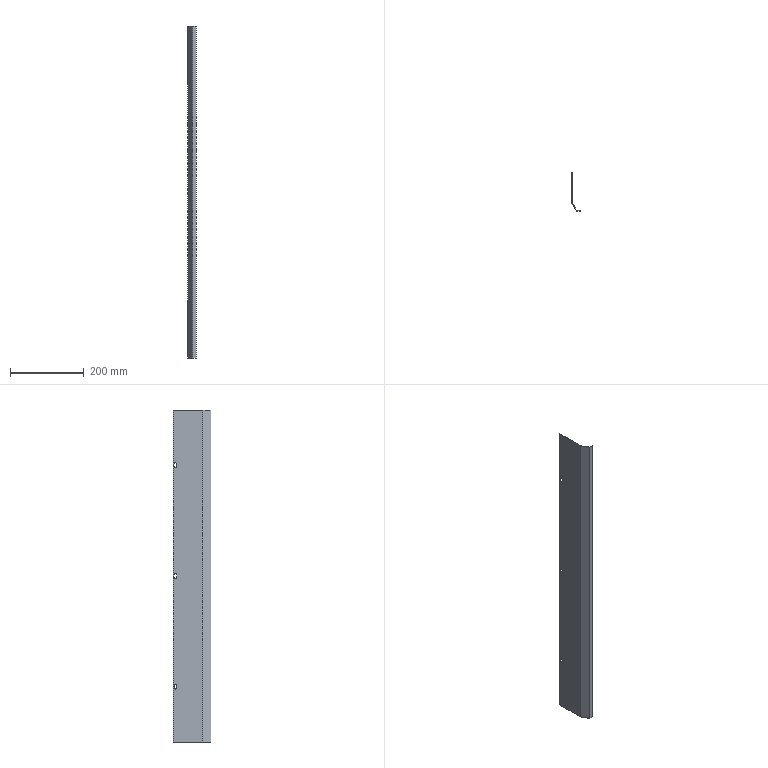Part | 1 solid | 37 faces | box 23.5 x 102.651 x 900 mm | volume 103908 mm3 | plane 24 | cylinder 13 | commonest cylinder face diameters 7 x6 6 x3 1 x2 3 x2
STEP:
#1=CARTESIAN_POINT('',(0.,-3.,-296.5));
#2=VERTEX_POINT('',#1);
#3=CARTESIAN_POINT('',(0.,-6.,-293.5));
#4=VERTEX_POINT('',#3);
#5=CARTESIAN_POINT('',(0.,-6.,-296.5));
#6=DIRECTION('',(1.,0.,0.));
#7=DIRECTION('',(0.,1.,0.));
#8=AXIS2_PLACEMENT_3D('',#5,#6,#7);
#9=CIRCLE('',#8,3.);
#10=EDGE_CURVE('',#2,#4,#9,.T.);
#11=ORIENTED_EDGE('',*,*,#10,.T.);
#12=CARTESIAN_POINT('',(-1.,-6.,-293.5));
#13=VERTEX_POINT('',#12);
#14=CARTESIAN_POINT('',(9.,-6.,-293.5));
#15=DIRECTION('',(-1.,0.,0.));
#16=VECTOR('',#15,1000.);
#17=LINE('',#14,#16);
#18=EDGE_CURVE('',#4,#13,#17,.T.);
#19=ORIENTED_EDGE('',*,*,#18,.T.);
#20=CARTESIAN_POINT('',(-1.,-3.,-296.5));
#21=VERTEX_POINT('',#20);
#22=CARTESIAN_POINT('',(-1.,-6.,-296.5));
#23=DIRECTION('',(-1.,0.,0.));
#24=DIRECTION('',(0.,0.,1.));
#25=AXIS2_PLACEMENT_3D('',#22,#23,#24);
#26=CIRCLE('',#25,3.);
#27=EDGE_CURVE('',#13,#21,#26,.T.);
#28=ORIENTED_EDGE('',*,*,#27,.T.);
#29=CARTESIAN_POINT('',(9.,-3.,-296.5));
#30=DIRECTION('',(-1.,0.,0.));
#31=VECTOR('',#30,1000.);
#32=LINE('',#29,#31);
#33=EDGE_CURVE('',#2,#21,#32,.T.);
#34=ORIENTED_EDGE('',*,*,#33,.F.);
#35=EDGE_LOOP('',(#11,#19,#28,#34));
#36=FACE_OUTER_BOUND('',#35,.T.);
#37=CARTESIAN_POINT('',(9.,-6.,-296.5));
#38=DIRECTION('',(-1.,0.,0.));
#39=DIRECTION('',(0.,0.,1.));
#40=AXIS2_PLACEMENT_3D('',#37,#38,#39);
#41=CYLINDRICAL_SURFACE('',#40,3.);
#42=ADVANCED_FACE('',(#36),#41,.F.);
#43=CARTESIAN_POINT('',(0.,-2.5,303.5));
#44=VERTEX_POINT('',#43);
#45=CARTESIAN_POINT('',(0.,-6.,307.));
#46=VERTEX_POINT('',#45);
#47=CARTESIAN_POINT('',(0.,-6.,303.5));
#48=DIRECTION('',(1.,0.,0.));
#49=DIRECTION('',(0.,1.,0.));
#50=AXIS2_PLACEMENT_3D('',#47,#48,#49);
#51=CIRCLE('',#50,3.5);
#52=EDGE_CURVE('',#44,#46,#51,.T.);
#53=ORIENTED_EDGE('',*,*,#52,.T.);
#54=CARTESIAN_POINT('',(-1.,-6.,307.));
#55=VERTEX_POINT('',#54);
#56=CARTESIAN_POINT('',(9.,-6.,307.));
#57=DIRECTION('',(-1.,0.,0.));
#58=VECTOR('',#57,1000.);
#59=LINE('',#56,#58);
#60=EDGE_CURVE('',#46,#55,#59,.T.);
#61=ORIENTED_EDGE('',*,*,#60,.T.);
#62=CARTESIAN_POINT('',(-1.,-2.5,303.5));
#63=VERTEX_POINT('',#62);
#64=CARTESIAN_POINT('',(-1.,-6.,303.5));
#65=DIRECTION('',(-1.,0.,0.));
#66=DIRECTION('',(0.,0.,1.));
#67=AXIS2_PLACEMENT_3D('',#64,#65,#66);
#68=CIRCLE('',#67,3.5);
#69=EDGE_CURVE('',#55,#63,#68,.T.);
#70=ORIENTED_EDGE('',*,*,#69,.T.);
#71=CARTESIAN_POINT('',(9.,-2.5,303.5));
#72=DIRECTION('',(-1.,0.,0.));
#73=VECTOR('',#72,1000.);
#74=LINE('',#71,#73);
#75=EDGE_CURVE('',#44,#63,#74,.T.);
#76=ORIENTED_EDGE('',*,*,#75,.F.);
#77=EDGE_LOOP('',(#53,#61,#70,#76));
#78=FACE_OUTER_BOUND('',#77,.T.);
#79=CARTESIAN_POINT('',(9.,-6.,303.5));
#80=DIRECTION('',(-1.,0.,0.));
#81=DIRECTION('',(0.,0.,1.));
#82=AXIS2_PLACEMENT_3D('',#79,#80,#81);
#83=CYLINDRICAL_SURFACE('',#82,3.5);
#84=ADVANCED_FACE('',(#78),#83,.F.);
#85=CARTESIAN_POINT('',(0.,-2.5,3.5));
#86=VERTEX_POINT('',#85);
#87=CARTESIAN_POINT('',(0.,-6.,7.));
#88=VERTEX_POINT('',#87);
#89=CARTESIAN_POINT('',(0.,-6.,3.5));
#90=DIRECTION('',(1.,0.,0.));
#91=DIRECTION('',(0.,1.,0.));
#92=AXIS2_PLACEMENT_3D('',#89,#90,#91);
#93=CIRCLE('',#92,3.5);
#94=EDGE_CURVE('',#86,#88,#93,.T.);
#95=ORIENTED_EDGE('',*,*,#94,.T.);
#96=CARTESIAN_POINT('',(-1.,-6.,7.));
#97=VERTEX_POINT('',#96);
#98=CARTESIAN_POINT('',(9.,-6.,7.));
#99=DIRECTION('',(-1.,0.,0.));
#100=VECTOR('',#99,1000.);
#101=LINE('',#98,#100);
#102=EDGE_CURVE('',#88,#97,#101,.T.);
#103=ORIENTED_EDGE('',*,*,#102,.T.);
#104=CARTESIAN_POINT('',(-1.,-2.5,3.5));
#105=VERTEX_POINT('',#104);
#106=CARTESIAN_POINT('',(-1.,-6.,3.5));
#107=DIRECTION('',(-1.,0.,0.));
#108=DIRECTION('',(0.,0.,1.));
#109=AXIS2_PLACEMENT_3D('',#106,#107,#108);
#110=CIRCLE('',#109,3.5);
#111=EDGE_CURVE('',#97,#105,#110,.T.);
#112=ORIENTED_EDGE('',*,*,#111,.T.);
#113=CARTESIAN_POINT('',(9.,-2.5,3.5));
#114=DIRECTION('',(-1.,0.,0.));
#115=VECTOR('',#114,1000.);
#116=LINE('',#113,#115);
#117=EDGE_CURVE('',#86,#105,#116,.T.);
#118=ORIENTED_EDGE('',*,*,#117,.F.);
#119=EDGE_LOOP('',(#95,#103,#112,#118));
#120=FACE_OUTER_BOUND('',#119,.T.);
#121=CARTESIAN_POINT('',(9.,-6.,3.5));
#122=DIRECTION('',(-1.,0.,0.));
#123=DIRECTION('',(0.,0.,1.));
#124=AXIS2_PLACEMENT_3D('',#121,#122,#123);
#125=CYLINDRICAL_SURFACE('',#124,3.5);
#126=ADVANCED_FACE('',(#120),#125,.F.);
#127=CARTESIAN_POINT('',(0.06699,-80.116,450.));
#128=VERTEX_POINT('',#127);
#129=CARTESIAN_POINT('',(-0.799,-80.616,450.));
#130=VERTEX_POINT('',#129);
#131=CARTESIAN_POINT('',(0.06699,-80.116,450.));
#132=DIRECTION('',(-0.866,-0.5,0.));
#133=VECTOR('',#132,1000.);
#134=LINE('',#131,#133);
#135=EDGE_CURVE('',#128,#130,#134,.T.);
#136=ORIENTED_EDGE('',*,*,#135,.F.);
#137=CARTESIAN_POINT('',(0.,-79.866,450.));
#138=VERTEX_POINT('',#137);
#139=CARTESIAN_POINT('',(0.5,-79.866,450.));
#140=DIRECTION('',(0.,0.,1.));
#141=DIRECTION('',(-1.,0.,0.));
#142=AXIS2_PLACEMENT_3D('',#139,#140,#141);
#143=CIRCLE('',#142,0.5);
#144=EDGE_CURVE('',#138,#128,#143,.T.);
#145=ORIENTED_EDGE('',*,*,#144,.F.);
#146=CARTESIAN_POINT('',(-1.,-79.866,450.));
#147=VERTEX_POINT('',#146);
#148=CARTESIAN_POINT('',(-1.,-79.866,450.));
#149=DIRECTION('',(1.,0.,0.));
#150=VECTOR('',#149,1000.);
#151=LINE('',#148,#150);
#152=EDGE_CURVE('',#147,#138,#151,.T.);
#153=ORIENTED_EDGE('',*,*,#152,.F.);
#154=CARTESIAN_POINT('',(0.5,-79.866,450.));
#155=DIRECTION('',(0.,0.,1.));
#156=DIRECTION('',(1.,0.,0.));
#157=AXIS2_PLACEMENT_3D('',#154,#155,#156);
#158=CIRCLE('',#157,1.5);
#159=EDGE_CURVE('',#147,#130,#158,.T.);
#160=ORIENTED_EDGE('',*,*,#159,.T.);
#161=EDGE_LOOP('',(#136,#145,#153,#160));
#162=FACE_OUTER_BOUND('',#161,.T.);
#163=CARTESIAN_POINT('',(0.06699,-80.116,450.));
#164=DIRECTION('',(0.,0.,1.));
#165=DIRECTION('',(1.,0.,0.));
#166=AXIS2_PLACEMENT_3D('',#163,#164,#165);
#167=PLANE('',#166);
#168=ADVANCED_FACE('',(#162),#167,.T.);
#169=CARTESIAN_POINT('',(12.356,-101.401,450.));
#170=VERTEX_POINT('',#169);
#171=CARTESIAN_POINT('',(0.,-80.,450.));
#172=DIRECTION('',(0.5,-0.866,0.));
#173=VECTOR('',#172,1000.);
#174=LINE('',#171,#173);
#175=EDGE_CURVE('',#128,#170,#174,.T.);
#176=ORIENTED_EDGE('',*,*,#175,.F.);
#177=ORIENTED_EDGE('',*,*,#135,.T.);
#178=CARTESIAN_POINT('',(11.49,-101.901,450.));
#179=VERTEX_POINT('',#178);
#180=CARTESIAN_POINT('',(-0.866,-80.5,450.));
#181=DIRECTION('',(0.5,-0.866,0.));
#182=VECTOR('',#181,1000.);
#183=LINE('',#180,#182);
#184=EDGE_CURVE('',#130,#179,#183,.T.);
#185=ORIENTED_EDGE('',*,*,#184,.T.);
#186=CARTESIAN_POINT('',(11.49,-101.901,450.));
#187=DIRECTION('',(0.866,0.5,0.));
#188=VECTOR('',#187,1000.);
#189=LINE('',#186,#188);
#190=EDGE_CURVE('',#179,#170,#189,.T.);
#191=ORIENTED_EDGE('',*,*,#190,.T.);
#192=EDGE_LOOP('',(#176,#177,#185,#191));
#193=FACE_OUTER_BOUND('',#192,.T.);
#194=CARTESIAN_POINT('',(-1.,-79.866,450.));
#195=DIRECTION('',(0.,0.,1.));
#196=DIRECTION('',(1.,0.,0.));
#197=AXIS2_PLACEMENT_3D('',#194,#195,#196);
#198=PLANE('',#197);
#199=ADVANCED_FACE('',(#193),#198,.T.);
#200=CARTESIAN_POINT('',(0.,-79.866,-450.));
#201=VERTEX_POINT('',#200);
#202=CARTESIAN_POINT('',(-1.,-79.866,-450.));
#203=VERTEX_POINT('',#202);
#204=CARTESIAN_POINT('',(0.,-79.866,-450.));
#205=DIRECTION('',(-1.,0.,0.));
#206=VECTOR('',#205,1000.);
#207=LINE('',#204,#206);
#208=EDGE_CURVE('',#201,#203,#207,.T.);
#209=ORIENTED_EDGE('',*,*,#208,.F.);
#210=CARTESIAN_POINT('',(0.06699,-80.116,-450.));
#211=VERTEX_POINT('',#210);
#212=CARTESIAN_POINT('',(0.5,-79.866,-450.));
#213=DIRECTION('',(0.,0.,1.));
#214=DIRECTION('',(-1.,0.,0.));
#215=AXIS2_PLACEMENT_3D('',#212,#213,#214);
#216=CIRCLE('',#215,0.5);
#217=EDGE_CURVE('',#201,#211,#216,.T.);
#218=ORIENTED_EDGE('',*,*,#217,.T.);
#219=CARTESIAN_POINT('',(-0.799,-80.616,-450.));
#220=VERTEX_POINT('',#219);
#221=CARTESIAN_POINT('',(-0.799,-80.616,-450.));
#222=DIRECTION('',(0.866,0.5,0.));
#223=VECTOR('',#222,1000.);
#224=LINE('',#221,#223);
#225=EDGE_CURVE('',#220,#211,#224,.T.);
#226=ORIENTED_EDGE('',*,*,#225,.F.);
#227=CARTESIAN_POINT('',(0.5,-79.866,-450.));
#228=DIRECTION('',(0.,0.,1.));
#229=DIRECTION('',(1.,0.,0.));
#230=AXIS2_PLACEMENT_3D('',#227,#228,#229);
#231=CIRCLE('',#230,1.5);
#232=EDGE_CURVE('',#203,#220,#231,.T.);
#233=ORIENTED_EDGE('',*,*,#232,.F.);
#234=EDGE_LOOP('',(#209,#218,#226,#233));
#235=FACE_OUTER_BOUND('',#234,.T.);
#236=CARTESIAN_POINT('',(0.,-79.866,-450.));
#237=DIRECTION('',(0.,0.,-1.));
#238=DIRECTION('',(-1.,0.,0.));
#239=AXIS2_PLACEMENT_3D('',#236,#237,#238);
#240=PLANE('',#239);
#241=ADVANCED_FACE('',(#235),#240,.T.);
#242=CARTESIAN_POINT('',(0.,0.,-450.));
#243=VERTEX_POINT('',#242);
#244=CARTESIAN_POINT('',(0.,0.,-450.));
#245=DIRECTION('',(0.,-1.,0.));
#246=VECTOR('',#245,1000.);
#247=LINE('',#244,#246);
#248=EDGE_CURVE('',#243,#201,#247,.T.);
#249=ORIENTED_EDGE('',*,*,#248,.T.);
#250=ORIENTED_EDGE('',*,*,#208,.T.);
#251=CARTESIAN_POINT('',(-1.,0.,-450.));
#252=VERTEX_POINT('',#251);
#253=CARTESIAN_POINT('',(-1.,0.,-450.));
#254=DIRECTION('',(0.,-1.,0.));
#255=VECTOR('',#254,1000.);
#256=LINE('',#253,#255);
#257=EDGE_CURVE('',#252,#203,#256,.T.);
#258=ORIENTED_EDGE('',*,*,#257,.F.);
#259=CARTESIAN_POINT('',(-1.,0.,-450.));
#260=DIRECTION('',(1.,0.,0.));
#261=VECTOR('',#260,1000.);
#262=LINE('',#259,#261);
#263=EDGE_CURVE('',#252,#243,#262,.T.);
#264=ORIENTED_EDGE('',*,*,#263,.T.);
#265=EDGE_LOOP('',(#249,#250,#258,#264));
#266=FACE_OUTER_BOUND('',#265,.T.);
#267=CARTESIAN_POINT('',(-0.799,-80.616,-450.));
#268=DIRECTION('',(0.,0.,-1.));
#269=DIRECTION('',(-1.,0.,0.));
#270=AXIS2_PLACEMENT_3D('',#267,#268,#269);
#271=PLANE('',#270);
#272=ADVANCED_FACE('',(#266),#271,.T.);
#273=CARTESIAN_POINT('',(12.789,-101.651,450.));
#274=VERTEX_POINT('',#273);
#275=CARTESIAN_POINT('',(12.789,-102.651,450.));
#276=VERTEX_POINT('',#275);
#277=CARTESIAN_POINT('',(12.789,-101.651,450.));
#278=DIRECTION('',(0.,-1.,0.));
#279=VECTOR('',#278,1000.);
#280=LINE('',#277,#279);
#281=EDGE_CURVE('',#274,#276,#280,.T.);
#282=ORIENTED_EDGE('',*,*,#281,.F.);
#283=CARTESIAN_POINT('',(12.789,-101.151,450.));
#284=DIRECTION('',(0.,0.,1.));
#285=DIRECTION('',(-1.,0.,0.));
#286=AXIS2_PLACEMENT_3D('',#283,#284,#285);
#287=CIRCLE('',#286,0.5);
#288=EDGE_CURVE('',#170,#274,#287,.T.);
#289=ORIENTED_EDGE('',*,*,#288,.F.);
#290=ORIENTED_EDGE('',*,*,#190,.F.);
#291=CARTESIAN_POINT('',(12.789,-101.151,450.));
#292=DIRECTION('',(0.,0.,1.));
#293=DIRECTION('',(1.,0.,0.));
#294=AXIS2_PLACEMENT_3D('',#291,#292,#293);
#295=CIRCLE('',#294,1.5);
#296=EDGE_CURVE('',#179,#276,#295,.T.);
#297=ORIENTED_EDGE('',*,*,#296,.T.);
#298=EDGE_LOOP('',(#282,#289,#290,#297));
#299=FACE_OUTER_BOUND('',#298,.T.);
#300=CARTESIAN_POINT('',(12.789,-101.651,450.));
#301=DIRECTION('',(0.,0.,1.));
#302=DIRECTION('',(1.,0.,0.));
#303=AXIS2_PLACEMENT_3D('',#300,#301,#302);
#304=PLANE('',#303);
#305=ADVANCED_FACE('',(#299),#304,.T.);
#306=CARTESIAN_POINT('',(22.5,-101.651,450.));
#307=VERTEX_POINT('',#306);
#308=CARTESIAN_POINT('',(12.5,-101.651,450.));
#309=DIRECTION('',(1.,0.,0.));
#310=VECTOR('',#309,1000.);
#311=LINE('',#308,#310);
#312=EDGE_CURVE('',#274,#307,#311,.T.);
#313=ORIENTED_EDGE('',*,*,#312,.F.);
#314=ORIENTED_EDGE('',*,*,#281,.T.);
#315=CARTESIAN_POINT('',(22.5,-102.651,450.));
#316=VERTEX_POINT('',#315);
#317=CARTESIAN_POINT('',(12.5,-102.651,450.));
#318=DIRECTION('',(1.,0.,0.));
#319=VECTOR('',#318,1000.);
#320=LINE('',#317,#319);
#321=EDGE_CURVE('',#276,#316,#320,.T.);
#322=ORIENTED_EDGE('',*,*,#321,.T.);
#323=CARTESIAN_POINT('',(22.5,-101.651,450.));
#324=DIRECTION('',(0.,-1.,0.));
#325=VECTOR('',#324,1000.);
#326=LINE('',#323,#325);
#327=EDGE_CURVE('',#307,#316,#326,.T.);
#328=ORIENTED_EDGE('',*,*,#327,.F.);
#329=EDGE_LOOP('',(#313,#314,#322,#328));
#330=FACE_OUTER_BOUND('',#329,.T.);
#331=CARTESIAN_POINT('',(11.49,-101.901,450.));
#332=DIRECTION('',(0.,0.,1.));
#333=DIRECTION('',(1.,0.,0.));
#334=AXIS2_PLACEMENT_3D('',#331,#332,#333);
#335=PLANE('',#334);
#336=ADVANCED_FACE('',(#330),#335,.T.);
#337=CARTESIAN_POINT('',(12.356,-101.401,-450.));
#338=VERTEX_POINT('',#337);
#339=CARTESIAN_POINT('',(11.49,-101.901,-450.));
#340=VERTEX_POINT('',#339);
#341=CARTESIAN_POINT('',(12.356,-101.401,-450.));
#342=DIRECTION('',(-0.866,-0.5,0.));
#343=VECTOR('',#342,1000.);
#344=LINE('',#341,#343);
#345=EDGE_CURVE('',#338,#340,#344,.T.);
#346=ORIENTED_EDGE('',*,*,#345,.F.);
#347=CARTESIAN_POINT('',(12.789,-101.651,-450.));
#348=VERTEX_POINT('',#347);
#349=CARTESIAN_POINT('',(12.789,-101.151,-450.));
#350=DIRECTION('',(0.,0.,1.));
#351=DIRECTION('',(-1.,0.,0.));
#352=AXIS2_PLACEMENT_3D('',#349,#350,#351);
#353=CIRCLE('',#352,0.5);
#354=EDGE_CURVE('',#338,#348,#353,.T.);
#355=ORIENTED_EDGE('',*,*,#354,.T.);
#356=CARTESIAN_POINT('',(12.789,-102.651,-450.));
#357=VERTEX_POINT('',#356);
#358=CARTESIAN_POINT('',(12.789,-102.651,-450.));
#359=DIRECTION('',(0.,1.,0.));
#360=VECTOR('',#359,1000.);
#361=LINE('',#358,#360);
#362=EDGE_CURVE('',#357,#348,#361,.T.);
#363=ORIENTED_EDGE('',*,*,#362,.F.);
#364=CARTESIAN_POINT('',(12.789,-101.151,-450.));
#365=DIRECTION('',(0.,0.,1.));
#366=DIRECTION('',(1.,0.,0.));
#367=AXIS2_PLACEMENT_3D('',#364,#365,#366);
#368=CIRCLE('',#367,1.5);
#369=EDGE_CURVE('',#340,#357,#368,.T.);
#370=ORIENTED_EDGE('',*,*,#369,.F.);
#371=EDGE_LOOP('',(#346,#355,#363,#370));
#372=FACE_OUTER_BOUND('',#371,.T.);
#373=CARTESIAN_POINT('',(12.356,-101.401,-450.));
#374=DIRECTION('',(0.,0.,-1.));
#375=DIRECTION('',(-1.,0.,0.));
#376=AXIS2_PLACEMENT_3D('',#373,#374,#375);
#377=PLANE('',#376);
#378=ADVANCED_FACE('',(#372),#377,.T.);
#379=CARTESIAN_POINT('',(0.,-80.,-450.));
#380=DIRECTION('',(0.5,-0.866,0.));
#381=VECTOR('',#380,1000.);
#382=LINE('',#379,#381);
#383=EDGE_CURVE('',#211,#338,#382,.T.);
#384=ORIENTED_EDGE('',*,*,#383,.T.);
#385=ORIENTED_EDGE('',*,*,#345,.T.);
#386=CARTESIAN_POINT('',(-0.866,-80.5,-450.));
#387=DIRECTION('',(0.5,-0.866,0.));
#388=VECTOR('',#387,1000.);
#389=LINE('',#386,#388);
#390=EDGE_CURVE('',#220,#340,#389,.T.);
#391=ORIENTED_EDGE('',*,*,#390,.F.);
#392=ORIENTED_EDGE('',*,*,#225,.T.);
#393=EDGE_LOOP('',(#384,#385,#391,#392));
#394=FACE_OUTER_BOUND('',#393,.T.);
#395=CARTESIAN_POINT('',(12.789,-102.651,-450.));
#396=DIRECTION('',(0.,0.,-1.));
#397=DIRECTION('',(-1.,0.,0.));
#398=AXIS2_PLACEMENT_3D('',#395,#396,#397);
#399=PLANE('',#398);
#400=ADVANCED_FACE('',(#394),#399,.T.);
#401=CARTESIAN_POINT('',(22.5,-102.651,-450.));
#402=VERTEX_POINT('',#401);
#403=CARTESIAN_POINT('',(12.5,-102.651,-450.));
#404=DIRECTION('',(1.,0.,0.));
#405=VECTOR('',#404,1000.);
#406=LINE('',#403,#405);
#407=EDGE_CURVE('',#357,#402,#406,.T.);
#408=ORIENTED_EDGE('',*,*,#407,.T.);
#409=CARTESIAN_POINT('',(22.5,-102.651,450.));
#410=DIRECTION('',(0.,0.,-1.));
#411=VECTOR('',#410,1000.);
#412=LINE('',#409,#411);
#413=EDGE_CURVE('',#316,#402,#412,.T.);
#414=ORIENTED_EDGE('',*,*,#413,.F.);
#415=ORIENTED_EDGE('',*,*,#321,.F.);
#416=CARTESIAN_POINT('',(12.789,-102.651,450.));
#417=DIRECTION('',(0.,0.,-1.));
#418=VECTOR('',#417,1000.);
#419=LINE('',#416,#418);
#420=EDGE_CURVE('',#276,#357,#419,.T.);
#421=ORIENTED_EDGE('',*,*,#420,.T.);
#422=EDGE_LOOP('',(#408,#414,#415,#421));
#423=FACE_OUTER_BOUND('',#422,.T.);
#424=CARTESIAN_POINT('',(12.5,-102.651,450.));
#425=DIRECTION('',(0.,1.,0.));
#426=DIRECTION('',(0.,0.,1.));
#427=AXIS2_PLACEMENT_3D('',#424,#425,#426);
#428=PLANE('',#427);
#429=ADVANCED_FACE('',(#423),#428,.F.);
#430=CARTESIAN_POINT('',(22.5,-101.651,-450.));
#431=VERTEX_POINT('',#430);
#432=CARTESIAN_POINT('',(22.5,-101.651,-450.));
#433=DIRECTION('',(0.,-1.,0.));
#434=VECTOR('',#433,1000.);
#435=LINE('',#432,#434);
#436=EDGE_CURVE('',#431,#402,#435,.T.);
#437=ORIENTED_EDGE('',*,*,#436,.F.);
#438=CARTESIAN_POINT('',(22.5,-101.651,450.));
#439=DIRECTION('',(0.,0.,-1.));
#440=VECTOR('',#439,1000.);
#441=LINE('',#438,#440);
#442=EDGE_CURVE('',#307,#431,#441,.T.);
#443=ORIENTED_EDGE('',*,*,#442,.F.);
#444=ORIENTED_EDGE('',*,*,#327,.T.);
#445=ORIENTED_EDGE('',*,*,#413,.T.);
#446=EDGE_LOOP('',(#437,#443,#444,#445));
#447=FACE_OUTER_BOUND('',#446,.T.);
#448=CARTESIAN_POINT('',(22.5,-101.651,450.));
#449=DIRECTION('',(1.,0.,0.));
#450=DIRECTION('',(0.,0.,-1.));
#451=AXIS2_PLACEMENT_3D('',#448,#449,#450);
#452=PLANE('',#451);
#453=ADVANCED_FACE('',(#447),#452,.T.);
#454=CARTESIAN_POINT('',(12.5,-101.651,-450.));
#455=DIRECTION('',(1.,0.,0.));
#456=VECTOR('',#455,1000.);
#457=LINE('',#454,#456);
#458=EDGE_CURVE('',#348,#431,#457,.T.);
#459=ORIENTED_EDGE('',*,*,#458,.F.);
#460=CARTESIAN_POINT('',(12.789,-101.651,450.));
#461=DIRECTION('',(0.,0.,-1.));
#462=VECTOR('',#461,1000.);
#463=LINE('',#460,#462);
#464=EDGE_CURVE('',#274,#348,#463,.T.);
#465=ORIENTED_EDGE('',*,*,#464,.F.);
#466=ORIENTED_EDGE('',*,*,#312,.T.);
#467=ORIENTED_EDGE('',*,*,#442,.T.);
#468=EDGE_LOOP('',(#459,#465,#466,#467));
#469=FACE_OUTER_BOUND('',#468,.T.);
#470=CARTESIAN_POINT('',(12.5,-101.651,450.));
#471=DIRECTION('',(0.,1.,0.));
#472=DIRECTION('',(0.,0.,1.));
#473=AXIS2_PLACEMENT_3D('',#470,#471,#472);
#474=PLANE('',#473);
#475=ADVANCED_FACE('',(#469),#474,.T.);
#476=ORIENTED_EDGE('',*,*,#354,.F.);
#477=CARTESIAN_POINT('',(12.356,-101.401,450.));
#478=DIRECTION('',(0.,0.,-1.));
#479=VECTOR('',#478,1000.);
#480=LINE('',#477,#479);
#481=EDGE_CURVE('',#170,#338,#480,.T.);
#482=ORIENTED_EDGE('',*,*,#481,.F.);
#483=ORIENTED_EDGE('',*,*,#288,.T.);
#484=ORIENTED_EDGE('',*,*,#464,.T.);
#485=EDGE_LOOP('',(#476,#482,#483,#484));
#486=FACE_OUTER_BOUND('',#485,.T.);
#487=CARTESIAN_POINT('',(12.789,-101.151,450.));
#488=DIRECTION('',(0.,0.,-1.));
#489=DIRECTION('',(-1.,0.,0.));
#490=AXIS2_PLACEMENT_3D('',#487,#488,#489);
#491=CYLINDRICAL_SURFACE('',#490,0.5);
#492=ADVANCED_FACE('',(#486),#491,.F.);
#493=ORIENTED_EDGE('',*,*,#383,.F.);
#494=CARTESIAN_POINT('',(0.06699,-80.116,450.));
#495=DIRECTION('',(0.,0.,-1.));
#496=VECTOR('',#495,1000.);
#497=LINE('',#494,#496);
#498=EDGE_CURVE('',#128,#211,#497,.T.);
#499=ORIENTED_EDGE('',*,*,#498,.F.);
#500=ORIENTED_EDGE('',*,*,#175,.T.);
#501=ORIENTED_EDGE('',*,*,#481,.T.);
#502=EDGE_LOOP('',(#493,#499,#500,#501));
#503=FACE_OUTER_BOUND('',#502,.T.);
#504=CARTESIAN_POINT('',(0.,-80.,450.));
#505=DIRECTION('',(0.866,0.5,0.));
#506=DIRECTION('',(-0.5,0.866,0.));
#507=AXIS2_PLACEMENT_3D('',#504,#505,#506);
#508=PLANE('',#507);
#509=ADVANCED_FACE('',(#503),#508,.T.);
#510=ORIENTED_EDGE('',*,*,#217,.F.);
#511=CARTESIAN_POINT('',(0.,-79.866,450.));
#512=DIRECTION('',(0.,0.,-1.));
#513=VECTOR('',#512,1000.);
#514=LINE('',#511,#513);
#515=EDGE_CURVE('',#138,#201,#514,.T.);
#516=ORIENTED_EDGE('',*,*,#515,.F.);
#517=ORIENTED_EDGE('',*,*,#144,.T.);
#518=ORIENTED_EDGE('',*,*,#498,.T.);
#519=EDGE_LOOP('',(#510,#516,#517,#518));
#520=FACE_OUTER_BOUND('',#519,.T.);
#521=CARTESIAN_POINT('',(0.5,-79.866,450.));
#522=DIRECTION('',(0.,0.,-1.));
#523=DIRECTION('',(-1.,0.,0.));
#524=AXIS2_PLACEMENT_3D('',#521,#522,#523);
#525=CYLINDRICAL_SURFACE('',#524,0.5);
#526=ADVANCED_FACE('',(#520),#525,.F.);
#527=CARTESIAN_POINT('',(0.,-9.,-303.5));
#528=VERTEX_POINT('',#527);
#529=CARTESIAN_POINT('',(0.,-3.,-303.5));
#530=VERTEX_POINT('',#529);
#531=CARTESIAN_POINT('',(0.,-6.,-303.5));
#532=DIRECTION('',(1.,0.,0.));
#533=DIRECTION('',(0.,1.,0.));
#534=AXIS2_PLACEMENT_3D('',#531,#532,#533);
#535=CIRCLE('',#534,3.);
#536=EDGE_CURVE('',#528,#530,#535,.T.);
#537=ORIENTED_EDGE('',*,*,#536,.F.);
#538=CARTESIAN_POINT('',(0.,-9.,-296.5));
#539=VERTEX_POINT('',#538);
#540=CARTESIAN_POINT('',(0.,-9.,450.));
#541=DIRECTION('',(0.,0.,-1.));
#542=VECTOR('',#541,1000.);
#543=LINE('',#540,#542);
#544=EDGE_CURVE('',#539,#528,#543,.T.);
#545=ORIENTED_EDGE('',*,*,#544,.F.);
#546=CARTESIAN_POINT('',(0.,-6.,-296.5));
#547=DIRECTION('',(1.,0.,0.));
#548=DIRECTION('',(0.,1.,0.));
#549=AXIS2_PLACEMENT_3D('',#546,#547,#548);
#550=CIRCLE('',#549,3.);
#551=EDGE_CURVE('',#4,#539,#550,.T.);
#552=ORIENTED_EDGE('',*,*,#551,.F.);
#553=ORIENTED_EDGE('',*,*,#10,.F.);
#554=CARTESIAN_POINT('',(0.,-3.,450.));
#555=DIRECTION('',(0.,0.,1.));
#556=VECTOR('',#555,1000.);
#557=LINE('',#554,#556);
#558=EDGE_CURVE('',#530,#2,#557,.T.);
#559=ORIENTED_EDGE('',*,*,#558,.F.);
#560=EDGE_LOOP('',(#537,#545,#552,#553,#559));
#561=FACE_BOUND('',#560,.T.);
#562=CARTESIAN_POINT('',(0.,-9.5,296.5));
#563=VERTEX_POINT('',#562);
#564=CARTESIAN_POINT('',(0.,-2.5,296.5));
#565=VERTEX_POINT('',#564);
#566=CARTESIAN_POINT('',(0.,-6.,296.5));
#567=DIRECTION('',(1.,0.,0.));
#568=DIRECTION('',(0.,1.,0.));
#569=AXIS2_PLACEMENT_3D('',#566,#567,#568);
#570=CIRCLE('',#569,3.5);
#571=EDGE_CURVE('',#563,#565,#570,.T.);
#572=ORIENTED_EDGE('',*,*,#571,.F.);
#573=CARTESIAN_POINT('',(0.,-9.5,303.5));
#574=VERTEX_POINT('',#573);
#575=CARTESIAN_POINT('',(0.,-9.5,450.));
#576=DIRECTION('',(0.,0.,-1.));
#577=VECTOR('',#576,1000.);
#578=LINE('',#575,#577);
#579=EDGE_CURVE('',#574,#563,#578,.T.);
#580=ORIENTED_EDGE('',*,*,#579,.F.);
#581=CARTESIAN_POINT('',(0.,-6.,303.5));
#582=DIRECTION('',(1.,0.,0.));
#583=DIRECTION('',(0.,1.,0.));
#584=AXIS2_PLACEMENT_3D('',#581,#582,#583);
#585=CIRCLE('',#584,3.5);
#586=EDGE_CURVE('',#46,#574,#585,.T.);
#587=ORIENTED_EDGE('',*,*,#586,.F.);
#588=ORIENTED_EDGE('',*,*,#52,.F.);
#589=CARTESIAN_POINT('',(0.,-2.5,450.));
#590=DIRECTION('',(0.,0.,1.));
#591=VECTOR('',#590,1000.);
#592=LINE('',#589,#591);
#593=EDGE_CURVE('',#565,#44,#592,.T.);
#594=ORIENTED_EDGE('',*,*,#593,.F.);
#595=EDGE_LOOP('',(#572,#580,#587,#588,#594));
#596=FACE_BOUND('',#595,.T.);
#597=CARTESIAN_POINT('',(0.,-9.5,-3.5));
#598=VERTEX_POINT('',#597);
#599=CARTESIAN_POINT('',(0.,-2.5,-3.5));
#600=VERTEX_POINT('',#599);
#601=CARTESIAN_POINT('',(0.,-6.,-3.5));
#602=DIRECTION('',(1.,0.,0.));
#603=DIRECTION('',(0.,1.,0.));
#604=AXIS2_PLACEMENT_3D('',#601,#602,#603);
#605=CIRCLE('',#604,3.5);
#606=EDGE_CURVE('',#598,#600,#605,.T.);
#607=ORIENTED_EDGE('',*,*,#606,.F.);
#608=CARTESIAN_POINT('',(0.,-9.5,3.5));
#609=VERTEX_POINT('',#608);
#610=CARTESIAN_POINT('',(0.,-9.5,450.));
#611=DIRECTION('',(0.,0.,-1.));
#612=VECTOR('',#611,1000.);
#613=LINE('',#610,#612);
#614=EDGE_CURVE('',#609,#598,#613,.T.);
#615=ORIENTED_EDGE('',*,*,#614,.F.);
#616=CARTESIAN_POINT('',(0.,-6.,3.5));
#617=DIRECTION('',(1.,0.,0.));
#618=DIRECTION('',(0.,1.,0.));
#619=AXIS2_PLACEMENT_3D('',#616,#617,#618);
#620=CIRCLE('',#619,3.5);
#621=EDGE_CURVE('',#88,#609,#620,.T.);
#622=ORIENTED_EDGE('',*,*,#621,.F.);
#623=ORIENTED_EDGE('',*,*,#94,.F.);
#624=CARTESIAN_POINT('',(0.,-2.5,450.));
#625=DIRECTION('',(0.,0.,1.));
#626=VECTOR('',#625,1000.);
#627=LINE('',#624,#626);
#628=EDGE_CURVE('',#600,#86,#627,.T.);
#629=ORIENTED_EDGE('',*,*,#628,.F.);
#630=EDGE_LOOP('',(#607,#615,#622,#623,#629));
#631=FACE_BOUND('',#630,.T.);
#632=ORIENTED_EDGE('',*,*,#248,.F.);
#633=CARTESIAN_POINT('',(0.,0.,450.));
#634=VERTEX_POINT('',#633);
#635=CARTESIAN_POINT('',(0.,0.,450.));
#636=DIRECTION('',(0.,0.,-1.));
#637=VECTOR('',#636,1000.);
#638=LINE('',#635,#637);
#639=EDGE_CURVE('',#634,#243,#638,.T.);
#640=ORIENTED_EDGE('',*,*,#639,.F.);
#641=CARTESIAN_POINT('',(0.,0.,450.));
#642=DIRECTION('',(0.,-1.,0.));
#643=VECTOR('',#642,1000.);
#644=LINE('',#641,#643);
#645=EDGE_CURVE('',#634,#138,#644,.T.);
#646=ORIENTED_EDGE('',*,*,#645,.T.);
#647=ORIENTED_EDGE('',*,*,#515,.T.);
#648=EDGE_LOOP('',(#632,#640,#646,#647));
#649=FACE_OUTER_BOUND('',#648,.T.);
#650=CARTESIAN_POINT('',(0.,0.,450.));
#651=DIRECTION('',(1.,0.,0.));
#652=DIRECTION('',(0.,1.,0.));
#653=AXIS2_PLACEMENT_3D('',#650,#651,#652);
#654=PLANE('',#653);
#655=ADVANCED_FACE('',(#561,#596,#631,#649),#654,.T.);
#656=ORIENTED_EDGE('',*,*,#263,.F.);
#657=CARTESIAN_POINT('',(-1.,0.,450.));
#658=VERTEX_POINT('',#657);
#659=CARTESIAN_POINT('',(-1.,0.,450.));
#660=DIRECTION('',(0.,0.,-1.));
#661=VECTOR('',#660,1000.);
#662=LINE('',#659,#661);
#663=EDGE_CURVE('',#658,#252,#662,.T.);
#664=ORIENTED_EDGE('',*,*,#663,.F.);
#665=CARTESIAN_POINT('',(-1.,0.,450.));
#666=DIRECTION('',(1.,0.,0.));
#667=VECTOR('',#666,1000.);
#668=LINE('',#665,#667);
#669=EDGE_CURVE('',#658,#634,#668,.T.);
#670=ORIENTED_EDGE('',*,*,#669,.T.);
#671=ORIENTED_EDGE('',*,*,#639,.T.);
#672=EDGE_LOOP('',(#656,#664,#670,#671));
#673=FACE_OUTER_BOUND('',#672,.T.);
#674=CARTESIAN_POINT('',(-1.,0.,450.));
#675=DIRECTION('',(0.,1.,0.));
#676=DIRECTION('',(-1.,0.,0.));
#677=AXIS2_PLACEMENT_3D('',#674,#675,#676);
#678=PLANE('',#677);
#679=ADVANCED_FACE('',(#673),#678,.T.);
#680=CARTESIAN_POINT('',(-1.,-9.,-303.5));
#681=VERTEX_POINT('',#680);
#682=CARTESIAN_POINT('',(-1.,-9.,-296.5));
#683=VERTEX_POINT('',#682);
#684=CARTESIAN_POINT('',(-1.,-9.,-303.5));
#685=DIRECTION('',(0.,0.,1.));
#686=VECTOR('',#685,1000.);
#687=LINE('',#684,#686);
#688=EDGE_CURVE('',#681,#683,#687,.T.);
#689=ORIENTED_EDGE('',*,*,#688,.F.);
#690=CARTESIAN_POINT('',(-1.,-3.,-303.5));
#691=VERTEX_POINT('',#690);
#692=CARTESIAN_POINT('',(-1.,-6.,-303.5));
#693=DIRECTION('',(-1.,0.,0.));
#694=DIRECTION('',(0.,0.,1.));
#695=AXIS2_PLACEMENT_3D('',#692,#693,#694);
#696=CIRCLE('',#695,3.);
#697=EDGE_CURVE('',#691,#681,#696,.T.);
#698=ORIENTED_EDGE('',*,*,#697,.F.);
#699=CARTESIAN_POINT('',(-1.,-3.,-303.5));
#700=DIRECTION('',(0.,0.,-1.));
#701=VECTOR('',#700,1000.);
#702=LINE('',#699,#701);
#703=EDGE_CURVE('',#21,#691,#702,.T.);
#704=ORIENTED_EDGE('',*,*,#703,.F.);
#705=ORIENTED_EDGE('',*,*,#27,.F.);
#706=CARTESIAN_POINT('',(-1.,-6.,-296.5));
#707=DIRECTION('',(-1.,0.,0.));
#708=DIRECTION('',(0.,0.,1.));
#709=AXIS2_PLACEMENT_3D('',#706,#707,#708);
#710=CIRCLE('',#709,3.);
#711=EDGE_CURVE('',#683,#13,#710,.T.);
#712=ORIENTED_EDGE('',*,*,#711,.F.);
#713=EDGE_LOOP('',(#689,#698,#704,#705,#712));
#714=FACE_BOUND('',#713,.T.);
#715=CARTESIAN_POINT('',(-1.,-9.5,296.5));
#716=VERTEX_POINT('',#715);
#717=CARTESIAN_POINT('',(-1.,-9.5,303.5));
#718=VERTEX_POINT('',#717);
#719=CARTESIAN_POINT('',(-1.,-9.5,296.5));
#720=DIRECTION('',(0.,0.,1.));
#721=VECTOR('',#720,1000.);
#722=LINE('',#719,#721);
#723=EDGE_CURVE('',#716,#718,#722,.T.);
#724=ORIENTED_EDGE('',*,*,#723,.F.);
#725=CARTESIAN_POINT('',(-1.,-2.5,296.5));
#726=VERTEX_POINT('',#725);
#727=CARTESIAN_POINT('',(-1.,-6.,296.5));
#728=DIRECTION('',(-1.,0.,0.));
#729=DIRECTION('',(0.,0.,1.));
#730=AXIS2_PLACEMENT_3D('',#727,#728,#729);
#731=CIRCLE('',#730,3.5);
#732=EDGE_CURVE('',#726,#716,#731,.T.);
#733=ORIENTED_EDGE('',*,*,#732,.F.);
#734=CARTESIAN_POINT('',(-1.,-2.5,296.5));
#735=DIRECTION('',(0.,0.,-1.));
#736=VECTOR('',#735,1000.);
#737=LINE('',#734,#736);
#738=EDGE_CURVE('',#63,#726,#737,.T.);
#739=ORIENTED_EDGE('',*,*,#738,.F.);
#740=ORIENTED_EDGE('',*,*,#69,.F.);
#741=CARTESIAN_POINT('',(-1.,-6.,303.5));
#742=DIRECTION('',(-1.,0.,0.));
#743=DIRECTION('',(0.,0.,1.));
#744=AXIS2_PLACEMENT_3D('',#741,#742,#743);
#745=CIRCLE('',#744,3.5);
#746=EDGE_CURVE('',#718,#55,#745,.T.);
#747=ORIENTED_EDGE('',*,*,#746,.F.);
#748=EDGE_LOOP('',(#724,#733,#739,#740,#747));
#749=FACE_BOUND('',#748,.T.);
#750=CARTESIAN_POINT('',(-1.,-9.5,-3.5));
#751=VERTEX_POINT('',#750);
#752=CARTESIAN_POINT('',(-1.,-9.5,3.5));
#753=VERTEX_POINT('',#752);
#754=CARTESIAN_POINT('',(-1.,-9.5,-3.5));
#755=DIRECTION('',(0.,0.,1.));
#756=VECTOR('',#755,1000.);
#757=LINE('',#754,#756);
#758=EDGE_CURVE('',#751,#753,#757,.T.);
#759=ORIENTED_EDGE('',*,*,#758,.F.);
#760=CARTESIAN_POINT('',(-1.,-2.5,-3.5));
#761=VERTEX_POINT('',#760);
#762=CARTESIAN_POINT('',(-1.,-6.,-3.5));
#763=DIRECTION('',(-1.,0.,0.));
#764=DIRECTION('',(0.,0.,1.));
#765=AXIS2_PLACEMENT_3D('',#762,#763,#764);
#766=CIRCLE('',#765,3.5);
#767=EDGE_CURVE('',#761,#751,#766,.T.);
#768=ORIENTED_EDGE('',*,*,#767,.F.);
#769=CARTESIAN_POINT('',(-1.,-2.5,-3.5));
#770=DIRECTION('',(0.,0.,-1.));
#771=VECTOR('',#770,1000.);
#772=LINE('',#769,#771);
#773=EDGE_CURVE('',#105,#761,#772,.T.);
#774=ORIENTED_EDGE('',*,*,#773,.F.);
#775=ORIENTED_EDGE('',*,*,#111,.F.);
#776=CARTESIAN_POINT('',(-1.,-6.,3.5));
#777=DIRECTION('',(-1.,0.,0.));
#778=DIRECTION('',(0.,0.,1.));
#779=AXIS2_PLACEMENT_3D('',#776,#777,#778);
#780=CIRCLE('',#779,3.5);
#781=EDGE_CURVE('',#753,#97,#780,.T.);
#782=ORIENTED_EDGE('',*,*,#781,.F.);
#783=EDGE_LOOP('',(#759,#768,#774,#775,#782));
#784=FACE_BOUND('',#783,.T.);
#785=ORIENTED_EDGE('',*,*,#257,.T.);
#786=CARTESIAN_POINT('',(-1.,-79.866,450.));
#787=DIRECTION('',(0.,0.,-1.));
#788=VECTOR('',#787,1000.);
#789=LINE('',#786,#788);
#790=EDGE_CURVE('',#147,#203,#789,.T.);
#791=ORIENTED_EDGE('',*,*,#790,.F.);
#792=CARTESIAN_POINT('',(-1.,0.,450.));
#793=DIRECTION('',(0.,-1.,0.));
#794=VECTOR('',#793,1000.);
#795=LINE('',#792,#794);
#796=EDGE_CURVE('',#658,#147,#795,.T.);
#797=ORIENTED_EDGE('',*,*,#796,.F.);
#798=ORIENTED_EDGE('',*,*,#663,.T.);
#799=EDGE_LOOP('',(#785,#791,#797,#798));
#800=FACE_OUTER_BOUND('',#799,.T.);
#801=CARTESIAN_POINT('',(-1.,0.,450.));
#802=DIRECTION('',(1.,0.,0.));
#803=DIRECTION('',(0.,1.,0.));
#804=AXIS2_PLACEMENT_3D('',#801,#802,#803);
#805=PLANE('',#804);
#806=ADVANCED_FACE('',(#714,#749,#784,#800),#805,.F.);
#807=ORIENTED_EDGE('',*,*,#232,.T.);
#808=CARTESIAN_POINT('',(-0.799,-80.616,450.));
#809=DIRECTION('',(0.,0.,-1.));
#810=VECTOR('',#809,1000.);
#811=LINE('',#808,#810);
#812=EDGE_CURVE('',#130,#220,#811,.T.);
#813=ORIENTED_EDGE('',*,*,#812,.F.);
#814=ORIENTED_EDGE('',*,*,#159,.F.);
#815=ORIENTED_EDGE('',*,*,#790,.T.);
#816=EDGE_LOOP('',(#807,#813,#814,#815));
#817=FACE_OUTER_BOUND('',#816,.T.);
#818=CARTESIAN_POINT('',(0.5,-79.866,450.));
#819=DIRECTION('',(0.,0.,-1.));
#820=DIRECTION('',(-1.,0.,0.));
#821=AXIS2_PLACEMENT_3D('',#818,#819,#820);
#822=CYLINDRICAL_SURFACE('',#821,1.5);
#823=ADVANCED_FACE('',(#817),#822,.T.);
#824=ORIENTED_EDGE('',*,*,#390,.T.);
#825=CARTESIAN_POINT('',(11.49,-101.901,450.));
#826=DIRECTION('',(0.,0.,-1.));
#827=VECTOR('',#826,1000.);
#828=LINE('',#825,#827);
#829=EDGE_CURVE('',#179,#340,#828,.T.);
#830=ORIENTED_EDGE('',*,*,#829,.F.);
#831=ORIENTED_EDGE('',*,*,#184,.F.);
#832=ORIENTED_EDGE('',*,*,#812,.T.);
#833=EDGE_LOOP('',(#824,#830,#831,#832));
#834=FACE_OUTER_BOUND('',#833,.T.);
#835=CARTESIAN_POINT('',(-0.866,-80.5,450.));
#836=DIRECTION('',(0.866,0.5,0.));
#837=DIRECTION('',(-0.5,0.866,0.));
#838=AXIS2_PLACEMENT_3D('',#835,#836,#837);
#839=PLANE('',#838);
#840=ADVANCED_FACE('',(#834),#839,.F.);
#841=ORIENTED_EDGE('',*,*,#369,.T.);
#842=ORIENTED_EDGE('',*,*,#420,.F.);
#843=ORIENTED_EDGE('',*,*,#296,.F.);
#844=ORIENTED_EDGE('',*,*,#829,.T.);
#845=EDGE_LOOP('',(#841,#842,#843,#844));
#846=FACE_OUTER_BOUND('',#845,.T.);
#847=CARTESIAN_POINT('',(12.789,-101.151,450.));
#848=DIRECTION('',(0.,0.,-1.));
#849=DIRECTION('',(-1.,0.,0.));
#850=AXIS2_PLACEMENT_3D('',#847,#848,#849);
#851=CYLINDRICAL_SURFACE('',#850,1.5);
#852=ADVANCED_FACE('',(#846),#851,.T.);
#853=ORIENTED_EDGE('',*,*,#796,.T.);
#854=ORIENTED_EDGE('',*,*,#152,.T.);
#855=ORIENTED_EDGE('',*,*,#645,.F.);
#856=ORIENTED_EDGE('',*,*,#669,.F.);
#857=EDGE_LOOP('',(#853,#854,#855,#856));
#858=FACE_OUTER_BOUND('',#857,.T.);
#859=CARTESIAN_POINT('',(12.789,-101.151,450.));
#860=DIRECTION('',(0.,0.,-1.));
#861=DIRECTION('',(-1.,0.,0.));
#862=AXIS2_PLACEMENT_3D('',#859,#860,#861);
#863=PLANE('',#862);
#864=ADVANCED_FACE('',(#858),#863,.F.);
#865=ORIENTED_EDGE('',*,*,#407,.F.);
#866=ORIENTED_EDGE('',*,*,#362,.T.);
#867=ORIENTED_EDGE('',*,*,#458,.T.);
#868=ORIENTED_EDGE('',*,*,#436,.T.);
#869=EDGE_LOOP('',(#865,#866,#867,#868));
#870=FACE_OUTER_BOUND('',#869,.T.);
#871=CARTESIAN_POINT('',(12.789,-101.151,-450.));
#872=DIRECTION('',(0.,0.,-1.));
#873=DIRECTION('',(-1.,0.,0.));
#874=AXIS2_PLACEMENT_3D('',#871,#872,#873);
#875=PLANE('',#874);
#876=ADVANCED_FACE('',(#870),#875,.T.);
#877=ORIENTED_EDGE('',*,*,#606,.T.);
#878=CARTESIAN_POINT('',(9.,-2.5,-3.5));
#879=DIRECTION('',(-1.,0.,0.));
#880=VECTOR('',#879,1000.);
#881=LINE('',#878,#880);
#882=EDGE_CURVE('',#600,#761,#881,.T.);
#883=ORIENTED_EDGE('',*,*,#882,.T.);
#884=ORIENTED_EDGE('',*,*,#767,.T.);
#885=CARTESIAN_POINT('',(9.,-9.5,-3.5));
#886=DIRECTION('',(-1.,0.,0.));
#887=VECTOR('',#886,1000.);
#888=LINE('',#885,#887);
#889=EDGE_CURVE('',#598,#751,#888,.T.);
#890=ORIENTED_EDGE('',*,*,#889,.F.);
#891=EDGE_LOOP('',(#877,#883,#884,#890));
#892=FACE_OUTER_BOUND('',#891,.T.);
#893=CARTESIAN_POINT('',(9.,-6.,-3.5));
#894=DIRECTION('',(-1.,0.,0.));
#895=DIRECTION('',(0.,0.,1.));
#896=AXIS2_PLACEMENT_3D('',#893,#894,#895);
#897=CYLINDRICAL_SURFACE('',#896,3.5);
#898=ADVANCED_FACE('',(#892),#897,.F.);
#899=ORIENTED_EDGE('',*,*,#628,.T.);
#900=ORIENTED_EDGE('',*,*,#117,.T.);
#901=ORIENTED_EDGE('',*,*,#773,.T.);
#902=ORIENTED_EDGE('',*,*,#882,.F.);
#903=EDGE_LOOP('',(#899,#900,#901,#902));
#904=FACE_OUTER_BOUND('',#903,.T.);
#905=CARTESIAN_POINT('',(9.,-2.5,-3.5));
#906=DIRECTION('',(0.,1.,0.));
#907=DIRECTION('',(0.,0.,1.));
#908=AXIS2_PLACEMENT_3D('',#905,#906,#907);
#909=PLANE('',#908);
#910=ADVANCED_FACE('',(#904),#909,.F.);
#911=ORIENTED_EDGE('',*,*,#102,.F.);
#912=ORIENTED_EDGE('',*,*,#621,.T.);
#913=CARTESIAN_POINT('',(9.,-9.5,3.5));
#914=DIRECTION('',(-1.,0.,0.));
#915=VECTOR('',#914,1000.);
#916=LINE('',#913,#915);
#917=EDGE_CURVE('',#609,#753,#916,.T.);
#918=ORIENTED_EDGE('',*,*,#917,.T.);
#919=ORIENTED_EDGE('',*,*,#781,.T.);
#920=EDGE_LOOP('',(#911,#912,#918,#919));
#921=FACE_OUTER_BOUND('',#920,.T.);
#922=CARTESIAN_POINT('',(9.,-6.,3.5));
#923=DIRECTION('',(-1.,0.,0.));
#924=DIRECTION('',(0.,0.,1.));
#925=AXIS2_PLACEMENT_3D('',#922,#923,#924);
#926=CYLINDRICAL_SURFACE('',#925,3.5);
#927=ADVANCED_FACE('',(#921),#926,.F.);
#928=ORIENTED_EDGE('',*,*,#614,.T.);
#929=ORIENTED_EDGE('',*,*,#889,.T.);
#930=ORIENTED_EDGE('',*,*,#758,.T.);
#931=ORIENTED_EDGE('',*,*,#917,.F.);
#932=EDGE_LOOP('',(#928,#929,#930,#931));
#933=FACE_OUTER_BOUND('',#932,.T.);
#934=CARTESIAN_POINT('',(9.,-9.5,-3.5));
#935=DIRECTION('',(0.,-1.,0.));
#936=DIRECTION('',(0.,0.,-1.));
#937=AXIS2_PLACEMENT_3D('',#934,#935,#936);
#938=PLANE('',#937);
#939=ADVANCED_FACE('',(#933),#938,.F.);
#940=ORIENTED_EDGE('',*,*,#571,.T.);
#941=CARTESIAN_POINT('',(9.,-2.5,296.5));
#942=DIRECTION('',(-1.,0.,0.));
#943=VECTOR('',#942,1000.);
#944=LINE('',#941,#943);
#945=EDGE_CURVE('',#565,#726,#944,.T.);
#946=ORIENTED_EDGE('',*,*,#945,.T.);
#947=ORIENTED_EDGE('',*,*,#732,.T.);
#948=CARTESIAN_POINT('',(9.,-9.5,296.5));
#949=DIRECTION('',(-1.,0.,0.));
#950=VECTOR('',#949,1000.);
#951=LINE('',#948,#950);
#952=EDGE_CURVE('',#563,#716,#951,.T.);
#953=ORIENTED_EDGE('',*,*,#952,.F.);
#954=EDGE_LOOP('',(#940,#946,#947,#953));
#955=FACE_OUTER_BOUND('',#954,.T.);
#956=CARTESIAN_POINT('',(9.,-6.,296.5));
#957=DIRECTION('',(-1.,0.,0.));
#958=DIRECTION('',(0.,0.,1.));
#959=AXIS2_PLACEMENT_3D('',#956,#957,#958);
#960=CYLINDRICAL_SURFACE('',#959,3.5);
#961=ADVANCED_FACE('',(#955),#960,.F.);
#962=ORIENTED_EDGE('',*,*,#593,.T.);
#963=ORIENTED_EDGE('',*,*,#75,.T.);
#964=ORIENTED_EDGE('',*,*,#738,.T.);
#965=ORIENTED_EDGE('',*,*,#945,.F.);
#966=EDGE_LOOP('',(#962,#963,#964,#965));
#967=FACE_OUTER_BOUND('',#966,.T.);
#968=CARTESIAN_POINT('',(9.,-2.5,296.5));
#969=DIRECTION('',(0.,1.,0.));
#970=DIRECTION('',(0.,0.,1.));
#971=AXIS2_PLACEMENT_3D('',#968,#969,#970);
#972=PLANE('',#971);
#973=ADVANCED_FACE('',(#967),#972,.F.);
#974=ORIENTED_EDGE('',*,*,#60,.F.);
#975=ORIENTED_EDGE('',*,*,#586,.T.);
#976=CARTESIAN_POINT('',(9.,-9.5,303.5));
#977=DIRECTION('',(-1.,0.,0.));
#978=VECTOR('',#977,1000.);
#979=LINE('',#976,#978);
#980=EDGE_CURVE('',#574,#718,#979,.T.);
#981=ORIENTED_EDGE('',*,*,#980,.T.);
#982=ORIENTED_EDGE('',*,*,#746,.T.);
#983=EDGE_LOOP('',(#974,#975,#981,#982));
#984=FACE_OUTER_BOUND('',#983,.T.);
#985=CARTESIAN_POINT('',(9.,-6.,303.5));
#986=DIRECTION('',(-1.,0.,0.));
#987=DIRECTION('',(0.,0.,1.));
#988=AXIS2_PLACEMENT_3D('',#985,#986,#987);
#989=CYLINDRICAL_SURFACE('',#988,3.5);
#990=ADVANCED_FACE('',(#984),#989,.F.);
#991=ORIENTED_EDGE('',*,*,#579,.T.);
#992=ORIENTED_EDGE('',*,*,#952,.T.);
#993=ORIENTED_EDGE('',*,*,#723,.T.);
#994=ORIENTED_EDGE('',*,*,#980,.F.);
#995=EDGE_LOOP('',(#991,#992,#993,#994));
#996=FACE_OUTER_BOUND('',#995,.T.);
#997=CARTESIAN_POINT('',(9.,-9.5,296.5));
#998=DIRECTION('',(0.,-1.,0.));
#999=DIRECTION('',(0.,0.,-1.));
#1000=AXIS2_PLACEMENT_3D('',#997,#998,#999);
#1001=PLANE('',#1000);
#1002=ADVANCED_FACE('',(#996),#1001,.F.);
#1003=ORIENTED_EDGE('',*,*,#536,.T.);
#1004=CARTESIAN_POINT('',(9.,-3.,-303.5));
#1005=DIRECTION('',(-1.,0.,0.));
#1006=VECTOR('',#1005,1000.);
#1007=LINE('',#1004,#1006);
#1008=EDGE_CURVE('',#530,#691,#1007,.T.);
#1009=ORIENTED_EDGE('',*,*,#1008,.T.);
#1010=ORIENTED_EDGE('',*,*,#697,.T.);
#1011=CARTESIAN_POINT('',(9.,-9.,-303.5));
#1012=DIRECTION('',(-1.,0.,0.));
#1013=VECTOR('',#1012,1000.);
#1014=LINE('',#1011,#1013);
#1015=EDGE_CURVE('',#528,#681,#1014,.T.);
#1016=ORIENTED_EDGE('',*,*,#1015,.F.);
#1017=EDGE_LOOP('',(#1003,#1009,#1010,#1016));
#1018=FACE_OUTER_BOUND('',#1017,.T.);
#1019=CARTESIAN_POINT('',(9.,-6.,-303.5));
#1020=DIRECTION('',(-1.,0.,0.));
#1021=DIRECTION('',(0.,0.,1.));
#1022=AXIS2_PLACEMENT_3D('',#1019,#1020,#1021);
#1023=CYLINDRICAL_SURFACE('',#1022,3.);
#1024=ADVANCED_FACE('',(#1018),#1023,.F.);
#1025=ORIENTED_EDGE('',*,*,#558,.T.);
#1026=ORIENTED_EDGE('',*,*,#33,.T.);
#1027=ORIENTED_EDGE('',*,*,#703,.T.);
#1028=ORIENTED_EDGE('',*,*,#1008,.F.);
#1029=EDGE_LOOP('',(#1025,#1026,#1027,#1028));
#1030=FACE_OUTER_BOUND('',#1029,.T.);
#1031=CARTESIAN_POINT('',(9.,-3.,-303.5));
#1032=DIRECTION('',(0.,1.,0.));
#1033=DIRECTION('',(0.,0.,1.));
#1034=AXIS2_PLACEMENT_3D('',#1031,#1032,#1033);
#1035=PLANE('',#1034);
#1036=ADVANCED_FACE('',(#1030),#1035,.F.);
#1037=ORIENTED_EDGE('',*,*,#18,.F.);
#1038=ORIENTED_EDGE('',*,*,#551,.T.);
#1039=CARTESIAN_POINT('',(9.,-9.,-296.5));
#1040=DIRECTION('',(-1.,0.,0.));
#1041=VECTOR('',#1040,1000.);
#1042=LINE('',#1039,#1041);
#1043=EDGE_CURVE('',#539,#683,#1042,.T.);
#1044=ORIENTED_EDGE('',*,*,#1043,.T.);
#1045=ORIENTED_EDGE('',*,*,#711,.T.);
#1046=EDGE_LOOP('',(#1037,#1038,#1044,#1045));
#1047=FACE_OUTER_BOUND('',#1046,.T.);
#1048=CARTESIAN_POINT('',(9.,-6.,-296.5));
#1049=DIRECTION('',(-1.,0.,0.));
#1050=DIRECTION('',(0.,0.,1.));
#1051=AXIS2_PLACEMENT_3D('',#1048,#1049,#1050);
#1052=CYLINDRICAL_SURFACE('',#1051,3.);
#1053=ADVANCED_FACE('',(#1047),#1052,.F.);
#1054=ORIENTED_EDGE('',*,*,#544,.T.);
#1055=ORIENTED_EDGE('',*,*,#1015,.T.);
#1056=ORIENTED_EDGE('',*,*,#688,.T.);
#1057=ORIENTED_EDGE('',*,*,#1043,.F.);
#1058=EDGE_LOOP('',(#1054,#1055,#1056,#1057));
#1059=FACE_OUTER_BOUND('',#1058,.T.);
#1060=CARTESIAN_POINT('',(9.,-9.,-303.5));
#1061=DIRECTION('',(0.,-1.,0.));
#1062=DIRECTION('',(0.,0.,-1.));
#1063=AXIS2_PLACEMENT_3D('',#1060,#1061,#1062);
#1064=PLANE('',#1063);
#1065=ADVANCED_FACE('',(#1059),#1064,.F.);
#1066=CLOSED_SHELL('',(#42,#84,#126,#168,#199,#241,#272,#305,#336,#378,#400,#429,#453,#475,#492,#509,#526,#655,#679,#806,#823,#840,#852,#864,#876,#898,#910,#927,#939,#961,#973,#990,#1002,#1024,#1036,#1053,#1065));
#1067=MANIFOLD_SOLID_BREP('',#1066);
#1068=CARTESIAN_POINT('',(0.,0.,0.));
#1069=DIRECTION('',(0.,0.,1.));
#1070=DIRECTION('',(1.,0.,0.));
#1071=AXIS2_PLACEMENT_3D('',#1068,#1069,#1070);
#1072=(LENGTH_UNIT()NAMED_UNIT(*)SI_UNIT(.MILLI.,.METRE.));
#1073=UNCERTAINTY_MEASURE_WITH_UNIT(LENGTH_MEASURE(0.00001),#1072,'','');
#1074=(NAMED_UNIT(*)PLANE_ANGLE_UNIT()SI_UNIT($,.RADIAN.));
#1075=(NAMED_UNIT(*)SI_UNIT($,.STERADIAN.)SOLID_ANGLE_UNIT());
#1076=(GEOMETRIC_REPRESENTATION_CONTEXT(3)GLOBAL_UNCERTAINTY_ASSIGNED_CONTEXT((#1073))GLOBAL_UNIT_ASSIGNED_CONTEXT((#1072,#1074,#1075))REPRESENTATION_CONTEXT('',''));
#1077=ADVANCED_BREP_SHAPE_REPRESENTATION('',(#1067,#1071),#1076);